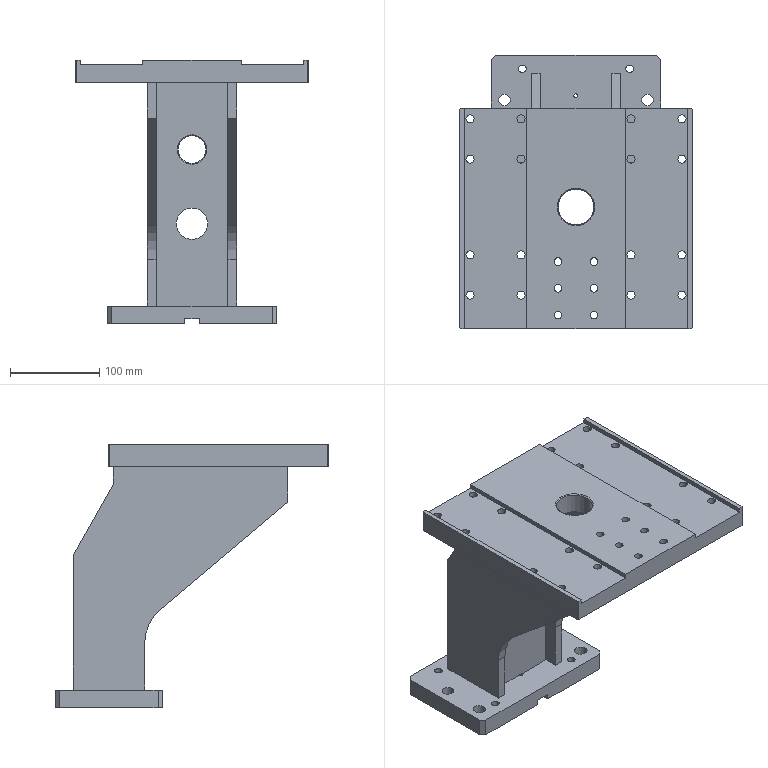Part | STEP file | YCD14007A-08.03.06 Clamping Arm (Left) | 1 solid | 133 faces | box 260 x 306 x 295 mm | volume 2759054 mm3 | cylinder 72 | plane 53 | cone 8 | commonest cylinder face diameters 9 x32 8.5 x20 4.2 x4 13 x4 14 x4 31 x2